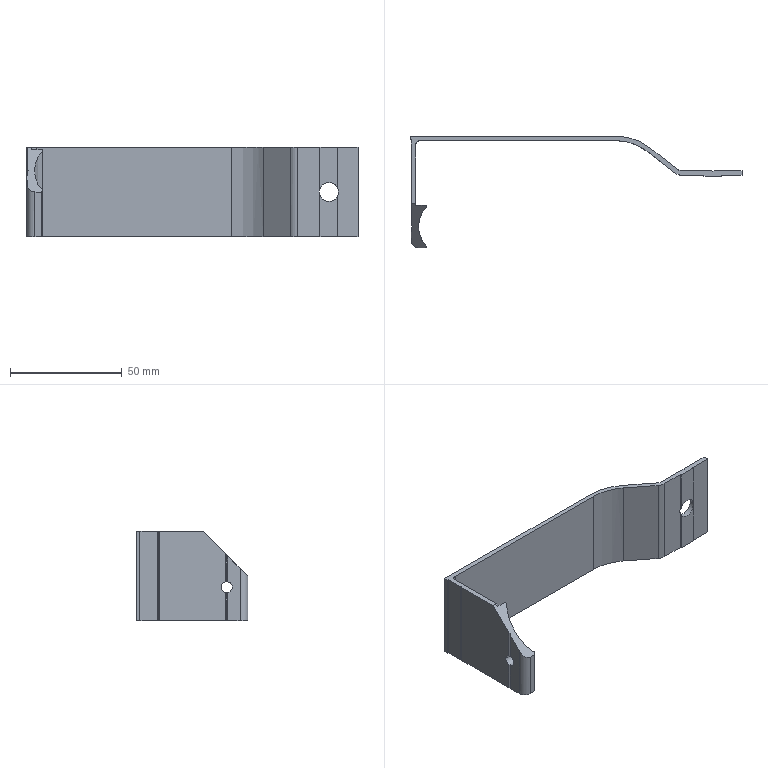Part | STEP file | 31E-01000QY15 | 1 solid | 52 faces | box 148.5 x 50 x 40 mm | volume 17043 mm3 | plane 36 | cylinder 16 | commonest cylinder face diameters 1 x4 5 x2 8.5 x2 25.4 x2 4 x1 6 x1